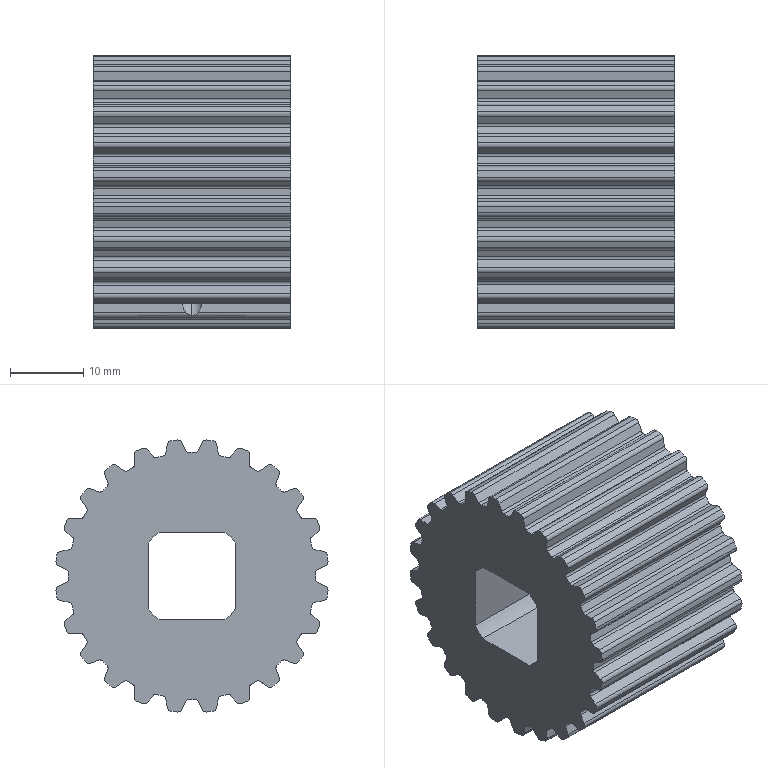Part | STEP file | TTPP24T5250-A-P11_b traction motor driven pulley | 1 solid | 216 faces | box 27 x 37.193 x 37.193 mm | volume 22972 mm3 | cylinder 158 | plane 58 | commonest cylinder face diameters 0.8 x52 1.2 x48 33.8 x26 37.4 x24 3.242 x4 15 x4